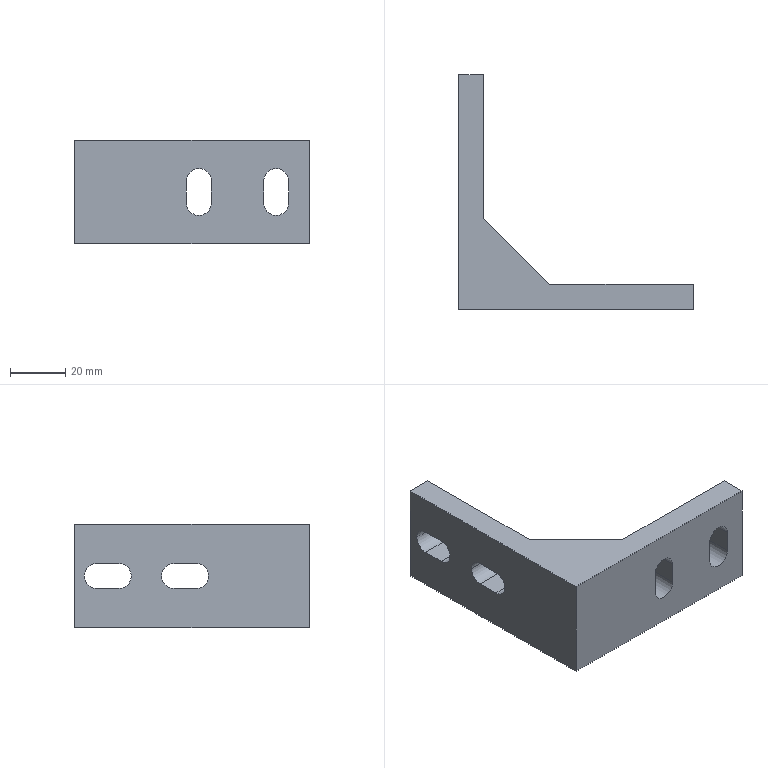Part | 1 solid | 29 faces | box 85 x 85 x 37.5 mm | volume 60255 mm3 | plane 17 | cylinder 12 | commonest cylinder face diameters 9 x12
STEP:
#1=CARTESIAN_POINT('',(30.5,-42.5,27.25));
#2=VERTEX_POINT('',#1);
#3=CARTESIAN_POINT('',(35.,-42.5,22.75));
#4=VERTEX_POINT('',#3);
#5=CARTESIAN_POINT('',(30.5,-42.5,22.75));
#6=DIRECTION('',(0.,1.,0.));
#7=DIRECTION('',(0.,0.,1.));
#8=AXIS2_PLACEMENT_3D('',#5,#6,#7);
#9=CIRCLE('',#8,4.5);
#10=EDGE_CURVE('',#2,#4,#9,.T.);
#11=ORIENTED_EDGE('',*,*,#10,.F.);
#12=CARTESIAN_POINT('',(30.5,-33.5,27.25));
#13=VERTEX_POINT('',#12);
#14=CARTESIAN_POINT('',(30.5,-42.5,27.25));
#15=DIRECTION('',(0.,1.,0.));
#16=VECTOR('',#15,1000.);
#17=LINE('',#14,#16);
#18=EDGE_CURVE('',#2,#13,#17,.T.);
#19=ORIENTED_EDGE('',*,*,#18,.T.);
#20=CARTESIAN_POINT('',(35.,-33.5,22.75));
#21=VERTEX_POINT('',#20);
#22=CARTESIAN_POINT('',(30.5,-33.5,22.75));
#23=DIRECTION('',(0.,1.,0.));
#24=DIRECTION('',(0.,0.,1.));
#25=AXIS2_PLACEMENT_3D('',#22,#23,#24);
#26=CIRCLE('',#25,4.5);
#27=EDGE_CURVE('',#13,#21,#26,.T.);
#28=ORIENTED_EDGE('',*,*,#27,.T.);
#29=CARTESIAN_POINT('',(35.,-42.5,22.75));
#30=DIRECTION('',(0.,1.,0.));
#31=VECTOR('',#30,1000.);
#32=LINE('',#29,#31);
#33=EDGE_CURVE('',#4,#21,#32,.T.);
#34=ORIENTED_EDGE('',*,*,#33,.F.);
#35=EDGE_LOOP('',(#11,#19,#28,#34));
#36=FACE_OUTER_BOUND('',#35,.T.);
#37=CARTESIAN_POINT('',(30.5,-42.5,22.75));
#38=DIRECTION('',(0.,1.,0.));
#39=DIRECTION('',(0.,0.,1.));
#40=AXIS2_PLACEMENT_3D('',#37,#38,#39);
#41=CYLINDRICAL_SURFACE('',#40,4.5);
#42=ADVANCED_FACE('',(#36),#41,.F.);
#43=CARTESIAN_POINT('',(2.5,-42.5,27.25));
#44=VERTEX_POINT('',#43);
#45=CARTESIAN_POINT('',(7.,-42.5,22.75));
#46=VERTEX_POINT('',#45);
#47=CARTESIAN_POINT('',(2.5,-42.5,22.75));
#48=DIRECTION('',(0.,1.,0.));
#49=DIRECTION('',(0.,0.,1.));
#50=AXIS2_PLACEMENT_3D('',#47,#48,#49);
#51=CIRCLE('',#50,4.5);
#52=EDGE_CURVE('',#44,#46,#51,.T.);
#53=ORIENTED_EDGE('',*,*,#52,.F.);
#54=CARTESIAN_POINT('',(2.5,-33.5,27.25));
#55=VERTEX_POINT('',#54);
#56=CARTESIAN_POINT('',(2.5,-42.5,27.25));
#57=DIRECTION('',(0.,1.,0.));
#58=VECTOR('',#57,1000.);
#59=LINE('',#56,#58);
#60=EDGE_CURVE('',#44,#55,#59,.T.);
#61=ORIENTED_EDGE('',*,*,#60,.T.);
#62=CARTESIAN_POINT('',(7.,-33.5,22.75));
#63=VERTEX_POINT('',#62);
#64=CARTESIAN_POINT('',(2.5,-33.5,22.75));
#65=DIRECTION('',(0.,1.,0.));
#66=DIRECTION('',(0.,0.,1.));
#67=AXIS2_PLACEMENT_3D('',#64,#65,#66);
#68=CIRCLE('',#67,4.5);
#69=EDGE_CURVE('',#55,#63,#68,.T.);
#70=ORIENTED_EDGE('',*,*,#69,.T.);
#71=CARTESIAN_POINT('',(7.,-42.5,22.75));
#72=DIRECTION('',(0.,1.,0.));
#73=VECTOR('',#72,1000.);
#74=LINE('',#71,#73);
#75=EDGE_CURVE('',#46,#63,#74,.T.);
#76=ORIENTED_EDGE('',*,*,#75,.F.);
#77=EDGE_LOOP('',(#53,#61,#70,#76));
#78=FACE_OUTER_BOUND('',#77,.T.);
#79=CARTESIAN_POINT('',(2.5,-42.5,22.75));
#80=DIRECTION('',(0.,1.,0.));
#81=DIRECTION('',(0.,0.,1.));
#82=AXIS2_PLACEMENT_3D('',#79,#80,#81);
#83=CYLINDRICAL_SURFACE('',#82,4.5);
#84=ADVANCED_FACE('',(#78),#83,.F.);
#85=CARTESIAN_POINT('',(-42.5,11.,18.75));
#86=VERTEX_POINT('',#85);
#87=CARTESIAN_POINT('',(-42.5,6.5,23.25));
#88=VERTEX_POINT('',#87);
#89=CARTESIAN_POINT('',(-42.5,6.5,18.75));
#90=DIRECTION('',(1.,0.,0.));
#91=DIRECTION('',(0.,1.,0.));
#92=AXIS2_PLACEMENT_3D('',#89,#90,#91);
#93=CIRCLE('',#92,4.5);
#94=EDGE_CURVE('',#86,#88,#93,.T.);
#95=ORIENTED_EDGE('',*,*,#94,.F.);
#96=CARTESIAN_POINT('',(-33.5,11.,18.75));
#97=VERTEX_POINT('',#96);
#98=CARTESIAN_POINT('',(-42.5,11.,18.75));
#99=DIRECTION('',(1.,0.,0.));
#100=VECTOR('',#99,1000.);
#101=LINE('',#98,#100);
#102=EDGE_CURVE('',#86,#97,#101,.T.);
#103=ORIENTED_EDGE('',*,*,#102,.T.);
#104=CARTESIAN_POINT('',(-33.5,6.5,23.25));
#105=VERTEX_POINT('',#104);
#106=CARTESIAN_POINT('',(-33.5,6.5,18.75));
#107=DIRECTION('',(1.,0.,0.));
#108=DIRECTION('',(0.,1.,0.));
#109=AXIS2_PLACEMENT_3D('',#106,#107,#108);
#110=CIRCLE('',#109,4.5);
#111=EDGE_CURVE('',#97,#105,#110,.T.);
#112=ORIENTED_EDGE('',*,*,#111,.T.);
#113=CARTESIAN_POINT('',(-42.5,6.5,23.25));
#114=DIRECTION('',(1.,0.,0.));
#115=VECTOR('',#114,1000.);
#116=LINE('',#113,#115);
#117=EDGE_CURVE('',#88,#105,#116,.T.);
#118=ORIENTED_EDGE('',*,*,#117,.F.);
#119=EDGE_LOOP('',(#95,#103,#112,#118));
#120=FACE_OUTER_BOUND('',#119,.T.);
#121=CARTESIAN_POINT('',(-42.5,6.5,18.75));
#122=DIRECTION('',(1.,0.,0.));
#123=DIRECTION('',(0.,1.,0.));
#124=AXIS2_PLACEMENT_3D('',#121,#122,#123);
#125=CYLINDRICAL_SURFACE('',#124,4.5);
#126=ADVANCED_FACE('',(#120),#125,.F.);
#127=CARTESIAN_POINT('',(-42.5,39.,18.75));
#128=VERTEX_POINT('',#127);
#129=CARTESIAN_POINT('',(-42.5,34.5,23.25));
#130=VERTEX_POINT('',#129);
#131=CARTESIAN_POINT('',(-42.5,34.5,18.75));
#132=DIRECTION('',(1.,0.,0.));
#133=DIRECTION('',(0.,1.,0.));
#134=AXIS2_PLACEMENT_3D('',#131,#132,#133);
#135=CIRCLE('',#134,4.5);
#136=EDGE_CURVE('',#128,#130,#135,.T.);
#137=ORIENTED_EDGE('',*,*,#136,.F.);
#138=CARTESIAN_POINT('',(-33.5,39.,18.75));
#139=VERTEX_POINT('',#138);
#140=CARTESIAN_POINT('',(-42.5,39.,18.75));
#141=DIRECTION('',(1.,0.,0.));
#142=VECTOR('',#141,1000.);
#143=LINE('',#140,#142);
#144=EDGE_CURVE('',#128,#139,#143,.T.);
#145=ORIENTED_EDGE('',*,*,#144,.T.);
#146=CARTESIAN_POINT('',(-33.5,34.5,23.25));
#147=VERTEX_POINT('',#146);
#148=CARTESIAN_POINT('',(-33.5,34.5,18.75));
#149=DIRECTION('',(1.,0.,0.));
#150=DIRECTION('',(0.,1.,0.));
#151=AXIS2_PLACEMENT_3D('',#148,#149,#150);
#152=CIRCLE('',#151,4.5);
#153=EDGE_CURVE('',#139,#147,#152,.T.);
#154=ORIENTED_EDGE('',*,*,#153,.T.);
#155=CARTESIAN_POINT('',(-42.5,34.5,23.25));
#156=DIRECTION('',(1.,0.,0.));
#157=VECTOR('',#156,1000.);
#158=LINE('',#155,#157);
#159=EDGE_CURVE('',#130,#147,#158,.T.);
#160=ORIENTED_EDGE('',*,*,#159,.F.);
#161=EDGE_LOOP('',(#137,#145,#154,#160));
#162=FACE_OUTER_BOUND('',#161,.T.);
#163=CARTESIAN_POINT('',(-42.5,34.5,18.75));
#164=DIRECTION('',(1.,0.,0.));
#165=DIRECTION('',(0.,1.,0.));
#166=AXIS2_PLACEMENT_3D('',#163,#164,#165);
#167=CYLINDRICAL_SURFACE('',#166,4.5);
#168=ADVANCED_FACE('',(#162),#167,.F.);
#169=CARTESIAN_POINT('',(-33.5,42.5,37.5));
#170=VERTEX_POINT('',#169);
#171=CARTESIAN_POINT('',(-33.5,42.5,0.));
#172=VERTEX_POINT('',#171);
#173=CARTESIAN_POINT('',(-33.5,42.5,37.5));
#174=DIRECTION('',(0.,0.,-1.));
#175=VECTOR('',#174,1000.);
#176=LINE('',#173,#175);
#177=EDGE_CURVE('',#170,#172,#176,.T.);
#178=ORIENTED_EDGE('',*,*,#177,.T.);
#179=CARTESIAN_POINT('',(-42.5,42.5,0.));
#180=VERTEX_POINT('',#179);
#181=CARTESIAN_POINT('',(42.5,42.5,0.));
#182=DIRECTION('',(-1.,0.,0.));
#183=VECTOR('',#182,1000.);
#184=LINE('',#181,#183);
#185=EDGE_CURVE('',#172,#180,#184,.T.);
#186=ORIENTED_EDGE('',*,*,#185,.T.);
#187=CARTESIAN_POINT('',(-42.5,42.5,37.5));
#188=VERTEX_POINT('',#187);
#189=CARTESIAN_POINT('',(-42.5,42.5,-37.5));
#190=DIRECTION('',(0.,0.,1.));
#191=VECTOR('',#190,1000.);
#192=LINE('',#189,#191);
#193=EDGE_CURVE('',#180,#188,#192,.T.);
#194=ORIENTED_EDGE('',*,*,#193,.T.);
#195=CARTESIAN_POINT('',(42.5,42.5,37.5));
#196=DIRECTION('',(-1.,0.,0.));
#197=VECTOR('',#196,1000.);
#198=LINE('',#195,#197);
#199=EDGE_CURVE('',#170,#188,#198,.T.);
#200=ORIENTED_EDGE('',*,*,#199,.F.);
#201=EDGE_LOOP('',(#178,#186,#194,#200));
#202=FACE_OUTER_BOUND('',#201,.T.);
#203=CARTESIAN_POINT('',(42.5,42.5,-37.5));
#204=DIRECTION('',(0.,1.,0.));
#205=DIRECTION('',(-1.,0.,0.));
#206=AXIS2_PLACEMENT_3D('',#203,#204,#205);
#207=PLANE('',#206);
#208=ADVANCED_FACE('',(#202),#207,.T.);
#209=CARTESIAN_POINT('',(42.5,-33.5,37.5));
#210=VERTEX_POINT('',#209);
#211=CARTESIAN_POINT('',(42.5,-33.5,0.));
#212=VERTEX_POINT('',#211);
#213=CARTESIAN_POINT('',(42.5,-33.5,37.5));
#214=DIRECTION('',(0.,0.,-1.));
#215=VECTOR('',#214,1000.);
#216=LINE('',#213,#215);
#217=EDGE_CURVE('',#210,#212,#216,.T.);
#218=ORIENTED_EDGE('',*,*,#217,.F.);
#219=CARTESIAN_POINT('',(42.5,-42.5,37.5));
#220=VERTEX_POINT('',#219);
#221=CARTESIAN_POINT('',(42.5,-42.5,37.5));
#222=DIRECTION('',(0.,1.,0.));
#223=VECTOR('',#222,1000.);
#224=LINE('',#221,#223);
#225=EDGE_CURVE('',#220,#210,#224,.T.);
#226=ORIENTED_EDGE('',*,*,#225,.F.);
#227=CARTESIAN_POINT('',(42.5,-42.5,0.));
#228=VERTEX_POINT('',#227);
#229=CARTESIAN_POINT('',(42.5,-42.5,-37.5));
#230=DIRECTION('',(0.,0.,1.));
#231=VECTOR('',#230,1000.);
#232=LINE('',#229,#231);
#233=EDGE_CURVE('',#228,#220,#232,.T.);
#234=ORIENTED_EDGE('',*,*,#233,.F.);
#235=CARTESIAN_POINT('',(42.5,-42.5,0.));
#236=DIRECTION('',(0.,1.,0.));
#237=VECTOR('',#236,1000.);
#238=LINE('',#235,#237);
#239=EDGE_CURVE('',#228,#212,#238,.T.);
#240=ORIENTED_EDGE('',*,*,#239,.T.);
#241=EDGE_LOOP('',(#218,#226,#234,#240));
#242=FACE_OUTER_BOUND('',#241,.T.);
#243=CARTESIAN_POINT('',(42.5,-42.5,-37.5));
#244=DIRECTION('',(1.,0.,0.));
#245=DIRECTION('',(0.,0.,-1.));
#246=AXIS2_PLACEMENT_3D('',#243,#244,#245);
#247=PLANE('',#246);
#248=ADVANCED_FACE('',(#242),#247,.T.);
#249=CARTESIAN_POINT('',(35.,-42.5,14.75));
#250=VERTEX_POINT('',#249);
#251=CARTESIAN_POINT('',(26.,-42.5,14.75));
#252=VERTEX_POINT('',#251);
#253=CARTESIAN_POINT('',(30.5,-42.5,14.75));
#254=DIRECTION('',(0.,1.,0.));
#255=DIRECTION('',(0.,0.,1.));
#256=AXIS2_PLACEMENT_3D('',#253,#254,#255);
#257=CIRCLE('',#256,4.5);
#258=EDGE_CURVE('',#250,#252,#257,.T.);
#259=ORIENTED_EDGE('',*,*,#258,.T.);
#260=CARTESIAN_POINT('',(26.,-42.5,22.75));
#261=VERTEX_POINT('',#260);
#262=CARTESIAN_POINT('',(26.,-42.5,22.75));
#263=DIRECTION('',(0.,0.,1.));
#264=VECTOR('',#263,1000.);
#265=LINE('',#262,#264);
#266=EDGE_CURVE('',#252,#261,#265,.T.);
#267=ORIENTED_EDGE('',*,*,#266,.T.);
#268=CARTESIAN_POINT('',(30.5,-42.5,22.75));
#269=DIRECTION('',(0.,1.,0.));
#270=DIRECTION('',(0.,0.,1.));
#271=AXIS2_PLACEMENT_3D('',#268,#269,#270);
#272=CIRCLE('',#271,4.5);
#273=EDGE_CURVE('',#261,#2,#272,.T.);
#274=ORIENTED_EDGE('',*,*,#273,.T.);
#275=ORIENTED_EDGE('',*,*,#10,.T.);
#276=CARTESIAN_POINT('',(35.,-42.5,14.75));
#277=DIRECTION('',(0.,0.,-1.));
#278=VECTOR('',#277,1000.);
#279=LINE('',#276,#278);
#280=EDGE_CURVE('',#4,#250,#279,.T.);
#281=ORIENTED_EDGE('',*,*,#280,.T.);
#282=EDGE_LOOP('',(#259,#267,#274,#275,#281));
#283=FACE_BOUND('',#282,.T.);
#284=CARTESIAN_POINT('',(-2.,-42.5,22.75));
#285=VERTEX_POINT('',#284);
#286=CARTESIAN_POINT('',(2.5,-42.5,22.75));
#287=DIRECTION('',(0.,1.,0.));
#288=DIRECTION('',(0.,0.,1.));
#289=AXIS2_PLACEMENT_3D('',#286,#287,#288);
#290=CIRCLE('',#289,4.5);
#291=EDGE_CURVE('',#285,#44,#290,.T.);
#292=ORIENTED_EDGE('',*,*,#291,.T.);
#293=ORIENTED_EDGE('',*,*,#52,.T.);
#294=CARTESIAN_POINT('',(7.,-42.5,14.75));
#295=VERTEX_POINT('',#294);
#296=CARTESIAN_POINT('',(7.,-42.5,22.75));
#297=DIRECTION('',(0.,0.,-1.));
#298=VECTOR('',#297,1000.);
#299=LINE('',#296,#298);
#300=EDGE_CURVE('',#46,#295,#299,.T.);
#301=ORIENTED_EDGE('',*,*,#300,.T.);
#302=CARTESIAN_POINT('',(-2.,-42.5,14.75));
#303=VERTEX_POINT('',#302);
#304=CARTESIAN_POINT('',(2.5,-42.5,14.75));
#305=DIRECTION('',(0.,1.,0.));
#306=DIRECTION('',(0.,0.,1.));
#307=AXIS2_PLACEMENT_3D('',#304,#305,#306);
#308=CIRCLE('',#307,4.5);
#309=EDGE_CURVE('',#295,#303,#308,.T.);
#310=ORIENTED_EDGE('',*,*,#309,.T.);
#311=CARTESIAN_POINT('',(-2.,-42.5,14.75));
#312=DIRECTION('',(0.,0.,1.));
#313=VECTOR('',#312,1000.);
#314=LINE('',#311,#313);
#315=EDGE_CURVE('',#303,#285,#314,.T.);
#316=ORIENTED_EDGE('',*,*,#315,.T.);
#317=EDGE_LOOP('',(#292,#293,#301,#310,#316));
#318=FACE_BOUND('',#317,.T.);
#319=CARTESIAN_POINT('',(-42.5,-42.5,37.5));
#320=VERTEX_POINT('',#319);
#321=CARTESIAN_POINT('',(-42.5,-42.5,37.5));
#322=DIRECTION('',(1.,0.,0.));
#323=VECTOR('',#322,1000.);
#324=LINE('',#321,#323);
#325=EDGE_CURVE('',#320,#220,#324,.T.);
#326=ORIENTED_EDGE('',*,*,#325,.F.);
#327=CARTESIAN_POINT('',(-42.5,-42.5,0.));
#328=VERTEX_POINT('',#327);
#329=CARTESIAN_POINT('',(-42.5,-42.5,-37.5));
#330=DIRECTION('',(0.,0.,1.));
#331=VECTOR('',#330,1000.);
#332=LINE('',#329,#331);
#333=EDGE_CURVE('',#328,#320,#332,.T.);
#334=ORIENTED_EDGE('',*,*,#333,.F.);
#335=CARTESIAN_POINT('',(-42.5,-42.5,0.));
#336=DIRECTION('',(1.,0.,0.));
#337=VECTOR('',#336,1000.);
#338=LINE('',#335,#337);
#339=EDGE_CURVE('',#328,#228,#338,.T.);
#340=ORIENTED_EDGE('',*,*,#339,.T.);
#341=ORIENTED_EDGE('',*,*,#233,.T.);
#342=EDGE_LOOP('',(#326,#334,#340,#341));
#343=FACE_OUTER_BOUND('',#342,.T.);
#344=CARTESIAN_POINT('',(-42.5,-42.5,-37.5));
#345=DIRECTION('',(0.,-1.,0.));
#346=DIRECTION('',(0.,0.,-1.));
#347=AXIS2_PLACEMENT_3D('',#344,#345,#346);
#348=PLANE('',#347);
#349=ADVANCED_FACE('',(#283,#318,#343),#348,.T.);
#350=CARTESIAN_POINT('',(-42.5,6.5,14.25));
#351=VERTEX_POINT('',#350);
#352=CARTESIAN_POINT('',(-42.5,6.5,18.75));
#353=DIRECTION('',(1.,0.,0.));
#354=DIRECTION('',(0.,1.,0.));
#355=AXIS2_PLACEMENT_3D('',#352,#353,#354);
#356=CIRCLE('',#355,4.5);
#357=EDGE_CURVE('',#351,#86,#356,.T.);
#358=ORIENTED_EDGE('',*,*,#357,.T.);
#359=ORIENTED_EDGE('',*,*,#94,.T.);
#360=CARTESIAN_POINT('',(-42.5,-1.5,23.25));
#361=VERTEX_POINT('',#360);
#362=CARTESIAN_POINT('',(-42.5,-1.5,23.25));
#363=DIRECTION('',(0.,-1.,0.));
#364=VECTOR('',#363,1000.);
#365=LINE('',#362,#364);
#366=EDGE_CURVE('',#88,#361,#365,.T.);
#367=ORIENTED_EDGE('',*,*,#366,.T.);
#368=CARTESIAN_POINT('',(-42.5,-1.5,14.25));
#369=VERTEX_POINT('',#368);
#370=CARTESIAN_POINT('',(-42.5,-1.5,18.75));
#371=DIRECTION('',(1.,0.,0.));
#372=DIRECTION('',(0.,1.,0.));
#373=AXIS2_PLACEMENT_3D('',#370,#371,#372);
#374=CIRCLE('',#373,4.5);
#375=EDGE_CURVE('',#361,#369,#374,.T.);
#376=ORIENTED_EDGE('',*,*,#375,.T.);
#377=CARTESIAN_POINT('',(-42.5,6.5,14.25));
#378=DIRECTION('',(0.,1.,0.));
#379=VECTOR('',#378,1000.);
#380=LINE('',#377,#379);
#381=EDGE_CURVE('',#369,#351,#380,.T.);
#382=ORIENTED_EDGE('',*,*,#381,.T.);
#383=EDGE_LOOP('',(#358,#359,#367,#376,#382));
#384=FACE_BOUND('',#383,.T.);
#385=CARTESIAN_POINT('',(-42.5,34.5,14.25));
#386=VERTEX_POINT('',#385);
#387=CARTESIAN_POINT('',(-42.5,34.5,18.75));
#388=DIRECTION('',(1.,0.,0.));
#389=DIRECTION('',(0.,1.,0.));
#390=AXIS2_PLACEMENT_3D('',#387,#388,#389);
#391=CIRCLE('',#390,4.5);
#392=EDGE_CURVE('',#386,#128,#391,.T.);
#393=ORIENTED_EDGE('',*,*,#392,.T.);
#394=ORIENTED_EDGE('',*,*,#136,.T.);
#395=CARTESIAN_POINT('',(-42.5,26.5,23.25));
#396=VERTEX_POINT('',#395);
#397=CARTESIAN_POINT('',(-42.5,26.5,23.25));
#398=DIRECTION('',(0.,-1.,0.));
#399=VECTOR('',#398,1000.);
#400=LINE('',#397,#399);
#401=EDGE_CURVE('',#130,#396,#400,.T.);
#402=ORIENTED_EDGE('',*,*,#401,.T.);
#403=CARTESIAN_POINT('',(-42.5,26.5,14.25));
#404=VERTEX_POINT('',#403);
#405=CARTESIAN_POINT('',(-42.5,26.5,18.75));
#406=DIRECTION('',(1.,0.,0.));
#407=DIRECTION('',(0.,1.,0.));
#408=AXIS2_PLACEMENT_3D('',#405,#406,#407);
#409=CIRCLE('',#408,4.5);
#410=EDGE_CURVE('',#396,#404,#409,.T.);
#411=ORIENTED_EDGE('',*,*,#410,.T.);
#412=CARTESIAN_POINT('',(-42.5,34.5,14.25));
#413=DIRECTION('',(0.,1.,0.));
#414=VECTOR('',#413,1000.);
#415=LINE('',#412,#414);
#416=EDGE_CURVE('',#404,#386,#415,.T.);
#417=ORIENTED_EDGE('',*,*,#416,.T.);
#418=EDGE_LOOP('',(#393,#394,#402,#411,#417));
#419=FACE_BOUND('',#418,.T.);
#420=CARTESIAN_POINT('',(-42.5,42.5,37.5));
#421=DIRECTION('',(0.,-1.,0.));
#422=VECTOR('',#421,1000.);
#423=LINE('',#420,#422);
#424=EDGE_CURVE('',#188,#320,#423,.T.);
#425=ORIENTED_EDGE('',*,*,#424,.F.);
#426=ORIENTED_EDGE('',*,*,#193,.F.);
#427=CARTESIAN_POINT('',(-42.5,42.5,0.));
#428=DIRECTION('',(0.,-1.,0.));
#429=VECTOR('',#428,1000.);
#430=LINE('',#427,#429);
#431=EDGE_CURVE('',#180,#328,#430,.T.);
#432=ORIENTED_EDGE('',*,*,#431,.T.);
#433=ORIENTED_EDGE('',*,*,#333,.T.);
#434=EDGE_LOOP('',(#425,#426,#432,#433));
#435=FACE_OUTER_BOUND('',#434,.T.);
#436=CARTESIAN_POINT('',(-42.5,42.5,-37.5));
#437=DIRECTION('',(-1.,0.,0.));
#438=DIRECTION('',(0.,-1.,0.));
#439=AXIS2_PLACEMENT_3D('',#436,#437,#438);
#440=PLANE('',#439);
#441=ADVANCED_FACE('',(#384,#419,#435),#440,.T.);
#442=ORIENTED_EDGE('',*,*,#185,.F.);
#443=CARTESIAN_POINT('',(-33.5,-9.5,0.));
#444=VERTEX_POINT('',#443);
#445=CARTESIAN_POINT('',(-33.5,-33.5,0.));
#446=DIRECTION('',(0.,1.,0.));
#447=VECTOR('',#446,1000.);
#448=LINE('',#445,#447);
#449=EDGE_CURVE('',#444,#172,#448,.T.);
#450=ORIENTED_EDGE('',*,*,#449,.F.);
#451=CARTESIAN_POINT('',(-9.5,-33.5,0.));
#452=VERTEX_POINT('',#451);
#453=CARTESIAN_POINT('',(-21.5,-21.5,0.));
#454=DIRECTION('',(0.7071,-0.7071,0.));
#455=VECTOR('',#454,1000.);
#456=LINE('',#453,#455);
#457=EDGE_CURVE('',#444,#452,#456,.T.);
#458=ORIENTED_EDGE('',*,*,#457,.T.);
#459=CARTESIAN_POINT('',(42.5,-33.5,0.));
#460=DIRECTION('',(-1.,0.,0.));
#461=VECTOR('',#460,1000.);
#462=LINE('',#459,#461);
#463=EDGE_CURVE('',#212,#452,#462,.T.);
#464=ORIENTED_EDGE('',*,*,#463,.F.);
#465=ORIENTED_EDGE('',*,*,#239,.F.);
#466=ORIENTED_EDGE('',*,*,#339,.F.);
#467=ORIENTED_EDGE('',*,*,#431,.F.);
#468=EDGE_LOOP('',(#442,#450,#458,#464,#465,#466,#467));
#469=FACE_OUTER_BOUND('',#468,.T.);
#470=CARTESIAN_POINT('',(0.,0.,0.));
#471=DIRECTION('',(0.,0.,1.));
#472=DIRECTION('',(1.,0.,0.));
#473=AXIS2_PLACEMENT_3D('',#470,#471,#472);
#474=PLANE('',#473);
#475=ADVANCED_FACE('',(#469),#474,.F.);
#476=CARTESIAN_POINT('',(-9.5,-33.5,37.5));
#477=VERTEX_POINT('',#476);
#478=CARTESIAN_POINT('',(42.5,-33.5,37.5));
#479=DIRECTION('',(-1.,0.,0.));
#480=VECTOR('',#479,1000.);
#481=LINE('',#478,#480);
#482=EDGE_CURVE('',#210,#477,#481,.T.);
#483=ORIENTED_EDGE('',*,*,#482,.T.);
#484=CARTESIAN_POINT('',(-33.5,-9.5,37.5));
#485=VERTEX_POINT('',#484);
#486=CARTESIAN_POINT('',(-33.5,-9.5,37.5));
#487=DIRECTION('',(-0.7071,0.7071,0.));
#488=VECTOR('',#487,1000.);
#489=LINE('',#486,#488);
#490=EDGE_CURVE('',#477,#485,#489,.T.);
#491=ORIENTED_EDGE('',*,*,#490,.T.);
#492=CARTESIAN_POINT('',(-33.5,-33.5,37.5));
#493=DIRECTION('',(0.,1.,0.));
#494=VECTOR('',#493,1000.);
#495=LINE('',#492,#494);
#496=EDGE_CURVE('',#485,#170,#495,.T.);
#497=ORIENTED_EDGE('',*,*,#496,.T.);
#498=ORIENTED_EDGE('',*,*,#199,.T.);
#499=ORIENTED_EDGE('',*,*,#424,.T.);
#500=ORIENTED_EDGE('',*,*,#325,.T.);
#501=ORIENTED_EDGE('',*,*,#225,.T.);
#502=EDGE_LOOP('',(#483,#491,#497,#498,#499,#500,#501));
#503=FACE_OUTER_BOUND('',#502,.T.);
#504=CARTESIAN_POINT('',(0.,0.,37.5));
#505=DIRECTION('',(0.,0.,1.));
#506=DIRECTION('',(1.,0.,0.));
#507=AXIS2_PLACEMENT_3D('',#504,#505,#506);
#508=PLANE('',#507);
#509=ADVANCED_FACE('',(#503),#508,.T.);
#510=CARTESIAN_POINT('',(-33.5,-1.5,23.25));
#511=VERTEX_POINT('',#510);
#512=CARTESIAN_POINT('',(-33.5,-1.5,23.25));
#513=DIRECTION('',(0.,-1.,0.));
#514=VECTOR('',#513,1000.);
#515=LINE('',#512,#514);
#516=EDGE_CURVE('',#105,#511,#515,.T.);
#517=ORIENTED_EDGE('',*,*,#516,.F.);
#518=ORIENTED_EDGE('',*,*,#111,.F.);
#519=CARTESIAN_POINT('',(-33.5,6.5,14.25));
#520=VERTEX_POINT('',#519);
#521=CARTESIAN_POINT('',(-33.5,6.5,18.75));
#522=DIRECTION('',(1.,0.,0.));
#523=DIRECTION('',(0.,1.,0.));
#524=AXIS2_PLACEMENT_3D('',#521,#522,#523);
#525=CIRCLE('',#524,4.5);
#526=EDGE_CURVE('',#520,#97,#525,.T.);
#527=ORIENTED_EDGE('',*,*,#526,.F.);
#528=CARTESIAN_POINT('',(-33.5,-1.5,14.25));
#529=VERTEX_POINT('',#528);
#530=CARTESIAN_POINT('',(-33.5,6.5,14.25));
#531=DIRECTION('',(0.,1.,0.));
#532=VECTOR('',#531,1000.);
#533=LINE('',#530,#532);
#534=EDGE_CURVE('',#529,#520,#533,.T.);
#535=ORIENTED_EDGE('',*,*,#534,.F.);
#536=CARTESIAN_POINT('',(-33.5,-1.5,18.75));
#537=DIRECTION('',(1.,0.,0.));
#538=DIRECTION('',(0.,1.,0.));
#539=AXIS2_PLACEMENT_3D('',#536,#537,#538);
#540=CIRCLE('',#539,4.5);
#541=EDGE_CURVE('',#511,#529,#540,.T.);
#542=ORIENTED_EDGE('',*,*,#541,.F.);
#543=EDGE_LOOP('',(#517,#518,#527,#535,#542));
#544=FACE_BOUND('',#543,.T.);
#545=CARTESIAN_POINT('',(-33.5,26.5,23.25));
#546=VERTEX_POINT('',#545);
#547=CARTESIAN_POINT('',(-33.5,26.5,23.25));
#548=DIRECTION('',(0.,-1.,0.));
#549=VECTOR('',#548,1000.);
#550=LINE('',#547,#549);
#551=EDGE_CURVE('',#147,#546,#550,.T.);
#552=ORIENTED_EDGE('',*,*,#551,.F.);
#553=ORIENTED_EDGE('',*,*,#153,.F.);
#554=CARTESIAN_POINT('',(-33.5,34.5,14.25));
#555=VERTEX_POINT('',#554);
#556=CARTESIAN_POINT('',(-33.5,34.5,18.75));
#557=DIRECTION('',(1.,0.,0.));
#558=DIRECTION('',(0.,1.,0.));
#559=AXIS2_PLACEMENT_3D('',#556,#557,#558);
#560=CIRCLE('',#559,4.5);
#561=EDGE_CURVE('',#555,#139,#560,.T.);
#562=ORIENTED_EDGE('',*,*,#561,.F.);
#563=CARTESIAN_POINT('',(-33.5,26.5,14.25));
#564=VERTEX_POINT('',#563);
#565=CARTESIAN_POINT('',(-33.5,34.5,14.25));
#566=DIRECTION('',(0.,1.,0.));
#567=VECTOR('',#566,1000.);
#568=LINE('',#565,#567);
#569=EDGE_CURVE('',#564,#555,#568,.T.);
#570=ORIENTED_EDGE('',*,*,#569,.F.);
#571=CARTESIAN_POINT('',(-33.5,26.5,18.75));
#572=DIRECTION('',(1.,0.,0.));
#573=DIRECTION('',(0.,1.,0.));
#574=AXIS2_PLACEMENT_3D('',#571,#572,#573);
#575=CIRCLE('',#574,4.5);
#576=EDGE_CURVE('',#546,#564,#575,.T.);
#577=ORIENTED_EDGE('',*,*,#576,.F.);
#578=EDGE_LOOP('',(#552,#553,#562,#570,#577));
#579=FACE_BOUND('',#578,.T.);
#580=ORIENTED_EDGE('',*,*,#496,.F.);
#581=CARTESIAN_POINT('',(-33.5,-9.5,-37.5));
#582=DIRECTION('',(0.,0.,-1.));
#583=VECTOR('',#582,1000.);
#584=LINE('',#581,#583);
#585=EDGE_CURVE('',#485,#444,#584,.T.);
#586=ORIENTED_EDGE('',*,*,#585,.T.);
#587=ORIENTED_EDGE('',*,*,#449,.T.);
#588=ORIENTED_EDGE('',*,*,#177,.F.);
#589=EDGE_LOOP('',(#580,#586,#587,#588));
#590=FACE_OUTER_BOUND('',#589,.T.);
#591=CARTESIAN_POINT('',(-33.5,-33.5,37.5));
#592=DIRECTION('',(-1.,0.,0.));
#593=DIRECTION('',(0.,-1.,0.));
#594=AXIS2_PLACEMENT_3D('',#591,#592,#593);
#595=PLANE('',#594);
#596=ADVANCED_FACE('',(#544,#579,#590),#595,.F.);
#597=CARTESIAN_POINT('',(26.,-33.5,14.75));
#598=VERTEX_POINT('',#597);
#599=CARTESIAN_POINT('',(26.,-33.5,22.75));
#600=VERTEX_POINT('',#599);
#601=CARTESIAN_POINT('',(26.,-33.5,22.75));
#602=DIRECTION('',(0.,0.,1.));
#603=VECTOR('',#602,1000.);
#604=LINE('',#601,#603);
#605=EDGE_CURVE('',#598,#600,#604,.T.);
#606=ORIENTED_EDGE('',*,*,#605,.F.);
#607=CARTESIAN_POINT('',(35.,-33.5,14.75));
#608=VERTEX_POINT('',#607);
#609=CARTESIAN_POINT('',(30.5,-33.5,14.75));
#610=DIRECTION('',(0.,1.,0.));
#611=DIRECTION('',(0.,0.,1.));
#612=AXIS2_PLACEMENT_3D('',#609,#610,#611);
#613=CIRCLE('',#612,4.5);
#614=EDGE_CURVE('',#608,#598,#613,.T.);
#615=ORIENTED_EDGE('',*,*,#614,.F.);
#616=CARTESIAN_POINT('',(35.,-33.5,14.75));
#617=DIRECTION('',(0.,0.,-1.));
#618=VECTOR('',#617,1000.);
#619=LINE('',#616,#618);
#620=EDGE_CURVE('',#21,#608,#619,.T.);
#621=ORIENTED_EDGE('',*,*,#620,.F.);
#622=ORIENTED_EDGE('',*,*,#27,.F.);
#623=CARTESIAN_POINT('',(30.5,-33.5,22.75));
#624=DIRECTION('',(0.,1.,0.));
#625=DIRECTION('',(0.,0.,1.));
#626=AXIS2_PLACEMENT_3D('',#623,#624,#625);
#627=CIRCLE('',#626,4.5);
#628=EDGE_CURVE('',#600,#13,#627,.T.);
#629=ORIENTED_EDGE('',*,*,#628,.F.);
#630=EDGE_LOOP('',(#606,#615,#621,#622,#629));
#631=FACE_BOUND('',#630,.T.);
#632=CARTESIAN_POINT('',(7.,-33.5,14.75));
#633=VERTEX_POINT('',#632);
#634=CARTESIAN_POINT('',(7.,-33.5,22.75));
#635=DIRECTION('',(0.,0.,-1.));
#636=VECTOR('',#635,1000.);
#637=LINE('',#634,#636);
#638=EDGE_CURVE('',#63,#633,#637,.T.);
#639=ORIENTED_EDGE('',*,*,#638,.F.);
#640=ORIENTED_EDGE('',*,*,#69,.F.);
#641=CARTESIAN_POINT('',(-2.,-33.5,22.75));
#642=VERTEX_POINT('',#641);
#643=CARTESIAN_POINT('',(2.5,-33.5,22.75));
#644=DIRECTION('',(0.,1.,0.));
#645=DIRECTION('',(0.,0.,1.));
#646=AXIS2_PLACEMENT_3D('',#643,#644,#645);
#647=CIRCLE('',#646,4.5);
#648=EDGE_CURVE('',#642,#55,#647,.T.);
#649=ORIENTED_EDGE('',*,*,#648,.F.);
#650=CARTESIAN_POINT('',(-2.,-33.5,14.75));
#651=VERTEX_POINT('',#650);
#652=CARTESIAN_POINT('',(-2.,-33.5,14.75));
#653=DIRECTION('',(0.,0.,1.));
#654=VECTOR('',#653,1000.);
#655=LINE('',#652,#654);
#656=EDGE_CURVE('',#651,#642,#655,.T.);
#657=ORIENTED_EDGE('',*,*,#656,.F.);
#658=CARTESIAN_POINT('',(2.5,-33.5,14.75));
#659=DIRECTION('',(0.,1.,0.));
#660=DIRECTION('',(0.,0.,1.));
#661=AXIS2_PLACEMENT_3D('',#658,#659,#660);
#662=CIRCLE('',#661,4.5);
#663=EDGE_CURVE('',#633,#651,#662,.T.);
#664=ORIENTED_EDGE('',*,*,#663,.F.);
#665=EDGE_LOOP('',(#639,#640,#649,#657,#664));
#666=FACE_BOUND('',#665,.T.);
#667=ORIENTED_EDGE('',*,*,#463,.T.);
#668=CARTESIAN_POINT('',(-9.5,-33.5,37.5));
#669=DIRECTION('',(0.,0.,1.));
#670=VECTOR('',#669,1000.);
#671=LINE('',#668,#670);
#672=EDGE_CURVE('',#452,#477,#671,.T.);
#673=ORIENTED_EDGE('',*,*,#672,.T.);
#674=ORIENTED_EDGE('',*,*,#482,.F.);
#675=ORIENTED_EDGE('',*,*,#217,.T.);
#676=EDGE_LOOP('',(#667,#673,#674,#675));
#677=FACE_OUTER_BOUND('',#676,.T.);
#678=CARTESIAN_POINT('',(42.5,-33.5,37.5));
#679=DIRECTION('',(0.,-1.,0.));
#680=DIRECTION('',(0.,0.,-1.));
#681=AXIS2_PLACEMENT_3D('',#678,#679,#680);
#682=PLANE('',#681);
#683=ADVANCED_FACE('',(#631,#666,#677),#682,.F.);
#684=ORIENTED_EDGE('',*,*,#490,.F.);
#685=ORIENTED_EDGE('',*,*,#672,.F.);
#686=ORIENTED_EDGE('',*,*,#457,.F.);
#687=ORIENTED_EDGE('',*,*,#585,.F.);
#688=EDGE_LOOP('',(#684,#685,#686,#687));
#689=FACE_OUTER_BOUND('',#688,.T.);
#690=CARTESIAN_POINT('',(-33.5,-9.5,37.5));
#691=DIRECTION('',(0.7071,0.7071,0.));
#692=DIRECTION('',(0.,0.,1.));
#693=AXIS2_PLACEMENT_3D('',#690,#691,#692);
#694=PLANE('',#693);
#695=ADVANCED_FACE('',(#689),#694,.T.);
#696=ORIENTED_EDGE('',*,*,#144,.F.);
#697=ORIENTED_EDGE('',*,*,#392,.F.);
#698=CARTESIAN_POINT('',(-42.5,34.5,14.25));
#699=DIRECTION('',(1.,0.,0.));
#700=VECTOR('',#699,1000.);
#701=LINE('',#698,#700);
#702=EDGE_CURVE('',#386,#555,#701,.T.);
#703=ORIENTED_EDGE('',*,*,#702,.T.);
#704=ORIENTED_EDGE('',*,*,#561,.T.);
#705=EDGE_LOOP('',(#696,#697,#703,#704));
#706=FACE_OUTER_BOUND('',#705,.T.);
#707=CARTESIAN_POINT('',(-42.5,34.5,18.75));
#708=DIRECTION('',(1.,0.,0.));
#709=DIRECTION('',(0.,1.,0.));
#710=AXIS2_PLACEMENT_3D('',#707,#708,#709);
#711=CYLINDRICAL_SURFACE('',#710,4.5);
#712=ADVANCED_FACE('',(#706),#711,.F.);
#713=ORIENTED_EDGE('',*,*,#569,.T.);
#714=ORIENTED_EDGE('',*,*,#702,.F.);
#715=ORIENTED_EDGE('',*,*,#416,.F.);
#716=CARTESIAN_POINT('',(-42.5,26.5,14.25));
#717=DIRECTION('',(1.,0.,0.));
#718=VECTOR('',#717,1000.);
#719=LINE('',#716,#718);
#720=EDGE_CURVE('',#404,#564,#719,.T.);
#721=ORIENTED_EDGE('',*,*,#720,.T.);
#722=EDGE_LOOP('',(#713,#714,#715,#721));
#723=FACE_OUTER_BOUND('',#722,.T.);
#724=CARTESIAN_POINT('',(-42.5,34.5,14.25));
#725=DIRECTION('',(0.,0.,-1.));
#726=DIRECTION('',(0.,1.,0.));
#727=AXIS2_PLACEMENT_3D('',#724,#725,#726);
#728=PLANE('',#727);
#729=ADVANCED_FACE('',(#723),#728,.F.);
#730=ORIENTED_EDGE('',*,*,#576,.T.);
#731=ORIENTED_EDGE('',*,*,#720,.F.);
#732=ORIENTED_EDGE('',*,*,#410,.F.);
#733=CARTESIAN_POINT('',(-42.5,26.5,23.25));
#734=DIRECTION('',(1.,0.,0.));
#735=VECTOR('',#734,1000.);
#736=LINE('',#733,#735);
#737=EDGE_CURVE('',#396,#546,#736,.T.);
#738=ORIENTED_EDGE('',*,*,#737,.T.);
#739=EDGE_LOOP('',(#730,#731,#732,#738));
#740=FACE_OUTER_BOUND('',#739,.T.);
#741=CARTESIAN_POINT('',(-42.5,26.5,18.75));
#742=DIRECTION('',(1.,0.,0.));
#743=DIRECTION('',(0.,1.,0.));
#744=AXIS2_PLACEMENT_3D('',#741,#742,#743);
#745=CYLINDRICAL_SURFACE('',#744,4.5);
#746=ADVANCED_FACE('',(#740),#745,.F.);
#747=ORIENTED_EDGE('',*,*,#551,.T.);
#748=ORIENTED_EDGE('',*,*,#737,.F.);
#749=ORIENTED_EDGE('',*,*,#401,.F.);
#750=ORIENTED_EDGE('',*,*,#159,.T.);
#751=EDGE_LOOP('',(#747,#748,#749,#750));
#752=FACE_OUTER_BOUND('',#751,.T.);
#753=CARTESIAN_POINT('',(-42.5,26.5,23.25));
#754=DIRECTION('',(0.,0.,1.));
#755=DIRECTION('',(1.,0.,0.));
#756=AXIS2_PLACEMENT_3D('',#753,#754,#755);
#757=PLANE('',#756);
#758=ADVANCED_FACE('',(#752),#757,.F.);
#759=ORIENTED_EDGE('',*,*,#102,.F.);
#760=ORIENTED_EDGE('',*,*,#357,.F.);
#761=CARTESIAN_POINT('',(-42.5,6.5,14.25));
#762=DIRECTION('',(1.,0.,0.));
#763=VECTOR('',#762,1000.);
#764=LINE('',#761,#763);
#765=EDGE_CURVE('',#351,#520,#764,.T.);
#766=ORIENTED_EDGE('',*,*,#765,.T.);
#767=ORIENTED_EDGE('',*,*,#526,.T.);
#768=EDGE_LOOP('',(#759,#760,#766,#767));
#769=FACE_OUTER_BOUND('',#768,.T.);
#770=CARTESIAN_POINT('',(-42.5,6.5,18.75));
#771=DIRECTION('',(1.,0.,0.));
#772=DIRECTION('',(0.,1.,0.));
#773=AXIS2_PLACEMENT_3D('',#770,#771,#772);
#774=CYLINDRICAL_SURFACE('',#773,4.5);
#775=ADVANCED_FACE('',(#769),#774,.F.);
#776=ORIENTED_EDGE('',*,*,#534,.T.);
#777=ORIENTED_EDGE('',*,*,#765,.F.);
#778=ORIENTED_EDGE('',*,*,#381,.F.);
#779=CARTESIAN_POINT('',(-42.5,-1.5,14.25));
#780=DIRECTION('',(1.,0.,0.));
#781=VECTOR('',#780,1000.);
#782=LINE('',#779,#781);
#783=EDGE_CURVE('',#369,#529,#782,.T.);
#784=ORIENTED_EDGE('',*,*,#783,.T.);
#785=EDGE_LOOP('',(#776,#777,#778,#784));
#786=FACE_OUTER_BOUND('',#785,.T.);
#787=CARTESIAN_POINT('',(-42.5,6.5,14.25));
#788=DIRECTION('',(0.,0.,-1.));
#789=DIRECTION('',(-1.,0.,0.));
#790=AXIS2_PLACEMENT_3D('',#787,#788,#789);
#791=PLANE('',#790);
#792=ADVANCED_FACE('',(#786),#791,.F.);
#793=ORIENTED_EDGE('',*,*,#541,.T.);
#794=ORIENTED_EDGE('',*,*,#783,.F.);
#795=ORIENTED_EDGE('',*,*,#375,.F.);
#796=CARTESIAN_POINT('',(-42.5,-1.5,23.25));
#797=DIRECTION('',(1.,0.,0.));
#798=VECTOR('',#797,1000.);
#799=LINE('',#796,#798);
#800=EDGE_CURVE('',#361,#511,#799,.T.);
#801=ORIENTED_EDGE('',*,*,#800,.T.);
#802=EDGE_LOOP('',(#793,#794,#795,#801));
#803=FACE_OUTER_BOUND('',#802,.T.);
#804=CARTESIAN_POINT('',(-42.5,-1.5,18.75));
#805=DIRECTION('',(1.,0.,0.));
#806=DIRECTION('',(0.,1.,0.));
#807=AXIS2_PLACEMENT_3D('',#804,#805,#806);
#808=CYLINDRICAL_SURFACE('',#807,4.5);
#809=ADVANCED_FACE('',(#803),#808,.F.);
#810=ORIENTED_EDGE('',*,*,#516,.T.);
#811=ORIENTED_EDGE('',*,*,#800,.F.);
#812=ORIENTED_EDGE('',*,*,#366,.F.);
#813=ORIENTED_EDGE('',*,*,#117,.T.);
#814=EDGE_LOOP('',(#810,#811,#812,#813));
#815=FACE_OUTER_BOUND('',#814,.T.);
#816=CARTESIAN_POINT('',(-42.5,-1.5,23.25));
#817=DIRECTION('',(0.,0.,1.));
#818=DIRECTION('',(0.,-1.,0.));
#819=AXIS2_PLACEMENT_3D('',#816,#817,#818);
#820=PLANE('',#819);
#821=ADVANCED_FACE('',(#815),#820,.F.);
#822=ORIENTED_EDGE('',*,*,#60,.F.);
#823=ORIENTED_EDGE('',*,*,#291,.F.);
#824=CARTESIAN_POINT('',(-2.,-42.5,22.75));
#825=DIRECTION('',(0.,1.,0.));
#826=VECTOR('',#825,1000.);
#827=LINE('',#824,#826);
#828=EDGE_CURVE('',#285,#642,#827,.T.);
#829=ORIENTED_EDGE('',*,*,#828,.T.);
#830=ORIENTED_EDGE('',*,*,#648,.T.);
#831=EDGE_LOOP('',(#822,#823,#829,#830));
#832=FACE_OUTER_BOUND('',#831,.T.);
#833=CARTESIAN_POINT('',(2.5,-42.5,22.75));
#834=DIRECTION('',(0.,1.,0.));
#835=DIRECTION('',(0.,0.,1.));
#836=AXIS2_PLACEMENT_3D('',#833,#834,#835);
#837=CYLINDRICAL_SURFACE('',#836,4.5);
#838=ADVANCED_FACE('',(#832),#837,.F.);
#839=ORIENTED_EDGE('',*,*,#656,.T.);
#840=ORIENTED_EDGE('',*,*,#828,.F.);
#841=ORIENTED_EDGE('',*,*,#315,.F.);
#842=CARTESIAN_POINT('',(-2.,-42.5,14.75));
#843=DIRECTION('',(0.,1.,0.));
#844=VECTOR('',#843,1000.);
#845=LINE('',#842,#844);
#846=EDGE_CURVE('',#303,#651,#845,.T.);
#847=ORIENTED_EDGE('',*,*,#846,.T.);
#848=EDGE_LOOP('',(#839,#840,#841,#847));
#849=FACE_OUTER_BOUND('',#848,.T.);
#850=CARTESIAN_POINT('',(-2.,-42.5,14.75));
#851=DIRECTION('',(-1.,0.,0.));
#852=DIRECTION('',(0.,0.,1.));
#853=AXIS2_PLACEMENT_3D('',#850,#851,#852);
#854=PLANE('',#853);
#855=ADVANCED_FACE('',(#849),#854,.F.);
#856=ORIENTED_EDGE('',*,*,#663,.T.);
#857=ORIENTED_EDGE('',*,*,#846,.F.);
#858=ORIENTED_EDGE('',*,*,#309,.F.);
#859=CARTESIAN_POINT('',(7.,-42.5,14.75));
#860=DIRECTION('',(0.,1.,0.));
#861=VECTOR('',#860,1000.);
#862=LINE('',#859,#861);
#863=EDGE_CURVE('',#295,#633,#862,.T.);
#864=ORIENTED_EDGE('',*,*,#863,.T.);
#865=EDGE_LOOP('',(#856,#857,#858,#864));
#866=FACE_OUTER_BOUND('',#865,.T.);
#867=CARTESIAN_POINT('',(2.5,-42.5,14.75));
#868=DIRECTION('',(0.,1.,0.));
#869=DIRECTION('',(0.,0.,1.));
#870=AXIS2_PLACEMENT_3D('',#867,#868,#869);
#871=CYLINDRICAL_SURFACE('',#870,4.5);
#872=ADVANCED_FACE('',(#866),#871,.F.);
#873=ORIENTED_EDGE('',*,*,#638,.T.);
#874=ORIENTED_EDGE('',*,*,#863,.F.);
#875=ORIENTED_EDGE('',*,*,#300,.F.);
#876=ORIENTED_EDGE('',*,*,#75,.T.);
#877=EDGE_LOOP('',(#873,#874,#875,#876));
#878=FACE_OUTER_BOUND('',#877,.T.);
#879=CARTESIAN_POINT('',(7.,-42.5,22.75));
#880=DIRECTION('',(1.,0.,0.));
#881=DIRECTION('',(0.,0.,-1.));
#882=AXIS2_PLACEMENT_3D('',#879,#880,#881);
#883=PLANE('',#882);
#884=ADVANCED_FACE('',(#878),#883,.F.);
#885=ORIENTED_EDGE('',*,*,#614,.T.);
#886=CARTESIAN_POINT('',(26.,-42.5,14.75));
#887=DIRECTION('',(0.,1.,0.));
#888=VECTOR('',#887,1000.);
#889=LINE('',#886,#888);
#890=EDGE_CURVE('',#252,#598,#889,.T.);
#891=ORIENTED_EDGE('',*,*,#890,.F.);
#892=ORIENTED_EDGE('',*,*,#258,.F.);
#893=CARTESIAN_POINT('',(35.,-42.5,14.75));
#894=DIRECTION('',(0.,1.,0.));
#895=VECTOR('',#894,1000.);
#896=LINE('',#893,#895);
#897=EDGE_CURVE('',#250,#608,#896,.T.);
#898=ORIENTED_EDGE('',*,*,#897,.T.);
#899=EDGE_LOOP('',(#885,#891,#892,#898));
#900=FACE_OUTER_BOUND('',#899,.T.);
#901=CARTESIAN_POINT('',(30.5,-42.5,14.75));
#902=DIRECTION('',(0.,1.,0.));
#903=DIRECTION('',(0.,0.,1.));
#904=AXIS2_PLACEMENT_3D('',#901,#902,#903);
#905=CYLINDRICAL_SURFACE('',#904,4.5);
#906=ADVANCED_FACE('',(#900),#905,.F.);
#907=ORIENTED_EDGE('',*,*,#620,.T.);
#908=ORIENTED_EDGE('',*,*,#897,.F.);
#909=ORIENTED_EDGE('',*,*,#280,.F.);
#910=ORIENTED_EDGE('',*,*,#33,.T.);
#911=EDGE_LOOP('',(#907,#908,#909,#910));
#912=FACE_OUTER_BOUND('',#911,.T.);
#913=CARTESIAN_POINT('',(35.,-42.5,14.75));
#914=DIRECTION('',(1.,0.,0.));
#915=DIRECTION('',(0.,0.,-1.));
#916=AXIS2_PLACEMENT_3D('',#913,#914,#915);
#917=PLANE('',#916);
#918=ADVANCED_FACE('',(#912),#917,.F.);
#919=ORIENTED_EDGE('',*,*,#18,.F.);
#920=ORIENTED_EDGE('',*,*,#273,.F.);
#921=CARTESIAN_POINT('',(26.,-42.5,22.75));
#922=DIRECTION('',(0.,1.,0.));
#923=VECTOR('',#922,1000.);
#924=LINE('',#921,#923);
#925=EDGE_CURVE('',#261,#600,#924,.T.);
#926=ORIENTED_EDGE('',*,*,#925,.T.);
#927=ORIENTED_EDGE('',*,*,#628,.T.);
#928=EDGE_LOOP('',(#919,#920,#926,#927));
#929=FACE_OUTER_BOUND('',#928,.T.);
#930=CARTESIAN_POINT('',(30.5,-42.5,22.75));
#931=DIRECTION('',(0.,1.,0.));
#932=DIRECTION('',(0.,0.,1.));
#933=AXIS2_PLACEMENT_3D('',#930,#931,#932);
#934=CYLINDRICAL_SURFACE('',#933,4.5);
#935=ADVANCED_FACE('',(#929),#934,.F.);
#936=ORIENTED_EDGE('',*,*,#605,.T.);
#937=ORIENTED_EDGE('',*,*,#925,.F.);
#938=ORIENTED_EDGE('',*,*,#266,.F.);
#939=ORIENTED_EDGE('',*,*,#890,.T.);
#940=EDGE_LOOP('',(#936,#937,#938,#939));
#941=FACE_OUTER_BOUND('',#940,.T.);
#942=CARTESIAN_POINT('',(26.,-42.5,22.75));
#943=DIRECTION('',(-1.,0.,0.));
#944=DIRECTION('',(0.,0.,1.));
#945=AXIS2_PLACEMENT_3D('',#942,#943,#944);
#946=PLANE('',#945);
#947=ADVANCED_FACE('',(#941),#946,.F.);
#948=CLOSED_SHELL('',(#42,#84,#126,#168,#208,#248,#349,#441,#475,#509,#596,#683,#695,#712,#729,#746,#758,#775,#792,#809,#821,#838,#855,#872,#884,#906,#918,#935,#947));
#949=MANIFOLD_SOLID_BREP('',#948);
#950=CARTESIAN_POINT('',(0.,0.,0.));
#951=DIRECTION('',(0.,0.,1.));
#952=DIRECTION('',(1.,0.,0.));
#953=AXIS2_PLACEMENT_3D('',#950,#951,#952);
#954=(LENGTH_UNIT()NAMED_UNIT(*)SI_UNIT(.MILLI.,.METRE.));
#955=UNCERTAINTY_MEASURE_WITH_UNIT(LENGTH_MEASURE(0.00001),#954,'','');
#956=(NAMED_UNIT(*)PLANE_ANGLE_UNIT()SI_UNIT($,.RADIAN.));
#957=(NAMED_UNIT(*)SI_UNIT($,.STERADIAN.)SOLID_ANGLE_UNIT());
#958=(GEOMETRIC_REPRESENTATION_CONTEXT(3)GLOBAL_UNCERTAINTY_ASSIGNED_CONTEXT((#955))GLOBAL_UNIT_ASSIGNED_CONTEXT((#954,#956,#957))REPRESENTATION_CONTEXT('',''));
#959=ADVANCED_BREP_SHAPE_REPRESENTATION('',(#949,#953),#958);